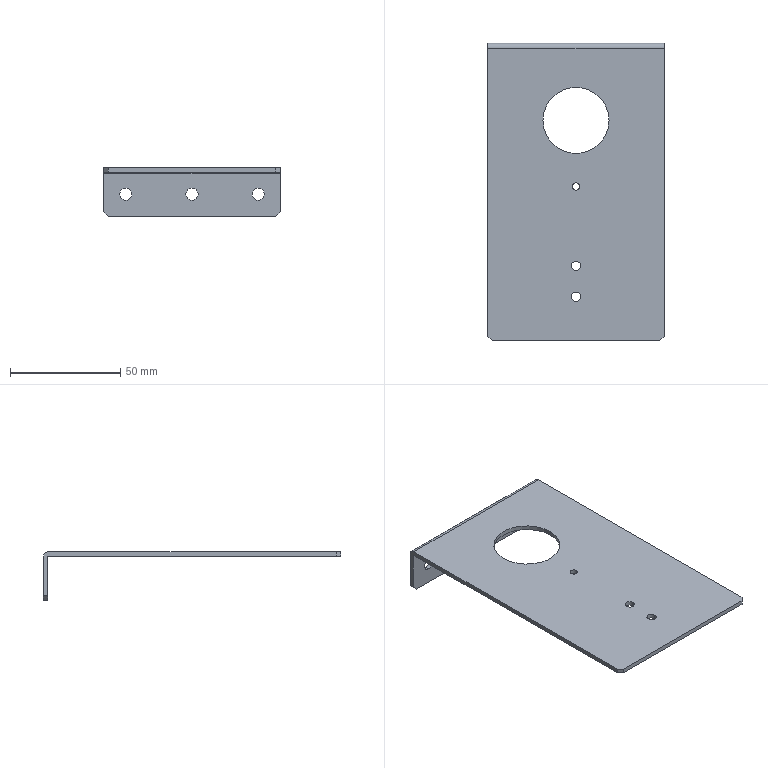Part | SolidWorks | features BaseBody 1 | 1 solid | 28 faces | box 80 x 135 x 22 mm | volume 23052 mm3 | cylinder 16 | plane 12 | commonest cylinder face diameters 5.5 x6 4.2 x4 3.3 x2 30 x2 1 x1 5 x1
STEP:
#1=CARTESIAN_POINT('',(37.9,34.,2.));
#2=VERTEX_POINT('',#1);
#3=CARTESIAN_POINT('',(42.1,34.,2.));
#4=VERTEX_POINT('',#3);
#5=CARTESIAN_POINT('',(40.,34.,2.));
#6=DIRECTION('',(0.,0.,1.));
#7=DIRECTION('',(-1.,0.,0.));
#8=AXIS2_PLACEMENT_3D('',#5,#6,#7);
#9=CIRCLE('',#8,2.1);
#10=EDGE_CURVE('',#2,#4,#9,.T.);
#11=ORIENTED_EDGE('',*,*,#10,.T.);
#12=CARTESIAN_POINT('',(42.1,34.,0.));
#13=VERTEX_POINT('',#12);
#14=CARTESIAN_POINT('',(42.1,34.,0.));
#15=DIRECTION('',(0.,0.,-1.));
#16=VECTOR('',#15,1000.);
#17=LINE('',#14,#16);
#18=EDGE_CURVE('',#4,#13,#17,.T.);
#19=ORIENTED_EDGE('',*,*,#18,.T.);
#20=CARTESIAN_POINT('',(37.9,34.,0.));
#21=VERTEX_POINT('',#20);
#22=CARTESIAN_POINT('',(40.,34.,0.));
#23=DIRECTION('',(0.,0.,1.));
#24=DIRECTION('',(-1.,0.,0.));
#25=AXIS2_PLACEMENT_3D('',#22,#23,#24);
#26=CIRCLE('',#25,2.1);
#27=EDGE_CURVE('',#21,#13,#26,.T.);
#28=ORIENTED_EDGE('',*,*,#27,.F.);
#29=CARTESIAN_POINT('',(37.9,34.,0.));
#30=DIRECTION('',(0.,0.,-1.));
#31=VECTOR('',#30,1000.);
#32=LINE('',#29,#31);
#33=EDGE_CURVE('',#2,#21,#32,.T.);
#34=ORIENTED_EDGE('',*,*,#33,.F.);
#35=EDGE_LOOP('',(#11,#19,#28,#34));
#36=FACE_OUTER_BOUND('',#35,.T.);
#37=CARTESIAN_POINT('',(40.,34.,0.));
#38=DIRECTION('',(0.,0.,-1.));
#39=DIRECTION('',(-1.,0.,0.));
#40=AXIS2_PLACEMENT_3D('',#37,#38,#39);
#41=CYLINDRICAL_SURFACE('',#40,2.1);
#42=ADVANCED_FACE('',(#36),#41,.F.);
#43=CARTESIAN_POINT('',(37.9,20.,2.));
#44=VERTEX_POINT('',#43);
#45=CARTESIAN_POINT('',(42.1,20.,2.));
#46=VERTEX_POINT('',#45);
#47=CARTESIAN_POINT('',(40.,20.,2.));
#48=DIRECTION('',(0.,0.,1.));
#49=DIRECTION('',(-1.,0.,0.));
#50=AXIS2_PLACEMENT_3D('',#47,#48,#49);
#51=CIRCLE('',#50,2.1);
#52=EDGE_CURVE('',#44,#46,#51,.T.);
#53=ORIENTED_EDGE('',*,*,#52,.T.);
#54=CARTESIAN_POINT('',(42.1,20.,0.));
#55=VERTEX_POINT('',#54);
#56=CARTESIAN_POINT('',(42.1,20.,0.));
#57=DIRECTION('',(0.,0.,-1.));
#58=VECTOR('',#57,1000.);
#59=LINE('',#56,#58);
#60=EDGE_CURVE('',#46,#55,#59,.T.);
#61=ORIENTED_EDGE('',*,*,#60,.T.);
#62=CARTESIAN_POINT('',(37.9,20.,0.));
#63=VERTEX_POINT('',#62);
#64=CARTESIAN_POINT('',(40.,20.,0.));
#65=DIRECTION('',(0.,0.,1.));
#66=DIRECTION('',(-1.,0.,0.));
#67=AXIS2_PLACEMENT_3D('',#64,#65,#66);
#68=CIRCLE('',#67,2.1);
#69=EDGE_CURVE('',#63,#55,#68,.T.);
#70=ORIENTED_EDGE('',*,*,#69,.F.);
#71=CARTESIAN_POINT('',(37.9,20.,0.));
#72=DIRECTION('',(0.,0.,-1.));
#73=VECTOR('',#72,1000.);
#74=LINE('',#71,#73);
#75=EDGE_CURVE('',#44,#63,#74,.T.);
#76=ORIENTED_EDGE('',*,*,#75,.F.);
#77=EDGE_LOOP('',(#53,#61,#70,#76));
#78=FACE_OUTER_BOUND('',#77,.T.);
#79=CARTESIAN_POINT('',(40.,20.,0.));
#80=DIRECTION('',(0.,0.,-1.));
#81=DIRECTION('',(-1.,0.,0.));
#82=AXIS2_PLACEMENT_3D('',#79,#80,#81);
#83=CYLINDRICAL_SURFACE('',#82,2.1);
#84=ADVANCED_FACE('',(#78),#83,.F.);
#85=CARTESIAN_POINT('',(25.,100.,2.));
#86=VERTEX_POINT('',#85);
#87=CARTESIAN_POINT('',(55.,100.,2.));
#88=VERTEX_POINT('',#87);
#89=CARTESIAN_POINT('',(40.,100.,2.));
#90=DIRECTION('',(0.,0.,1.));
#91=DIRECTION('',(-1.,0.,0.));
#92=AXIS2_PLACEMENT_3D('',#89,#90,#91);
#93=CIRCLE('',#92,15.);
#94=EDGE_CURVE('',#86,#88,#93,.T.);
#95=ORIENTED_EDGE('',*,*,#94,.T.);
#96=CARTESIAN_POINT('',(55.,100.,0.));
#97=VERTEX_POINT('',#96);
#98=CARTESIAN_POINT('',(55.,100.,10.));
#99=DIRECTION('',(0.,0.,-1.));
#100=VECTOR('',#99,1000.);
#101=LINE('',#98,#100);
#102=EDGE_CURVE('',#88,#97,#101,.T.);
#103=ORIENTED_EDGE('',*,*,#102,.T.);
#104=CARTESIAN_POINT('',(25.,100.,0.));
#105=VERTEX_POINT('',#104);
#106=CARTESIAN_POINT('',(40.,100.,0.));
#107=DIRECTION('',(0.,0.,1.));
#108=DIRECTION('',(-1.,0.,0.));
#109=AXIS2_PLACEMENT_3D('',#106,#107,#108);
#110=CIRCLE('',#109,15.);
#111=EDGE_CURVE('',#105,#97,#110,.T.);
#112=ORIENTED_EDGE('',*,*,#111,.F.);
#113=CARTESIAN_POINT('',(25.,100.,10.));
#114=DIRECTION('',(0.,0.,-1.));
#115=VECTOR('',#114,1000.);
#116=LINE('',#113,#115);
#117=EDGE_CURVE('',#86,#105,#116,.T.);
#118=ORIENTED_EDGE('',*,*,#117,.F.);
#119=EDGE_LOOP('',(#95,#103,#112,#118));
#120=FACE_OUTER_BOUND('',#119,.T.);
#121=CARTESIAN_POINT('',(40.,100.,10.));
#122=DIRECTION('',(0.,0.,-1.));
#123=DIRECTION('',(-1.,0.,0.));
#124=AXIS2_PLACEMENT_3D('',#121,#122,#123);
#125=CYLINDRICAL_SURFACE('',#124,15.);
#126=ADVANCED_FACE('',(#120),#125,.F.);
#127=CARTESIAN_POINT('',(38.35,70.,2.));
#128=VERTEX_POINT('',#127);
#129=CARTESIAN_POINT('',(41.65,70.,2.));
#130=VERTEX_POINT('',#129);
#131=CARTESIAN_POINT('',(40.,70.,2.));
#132=DIRECTION('',(0.,0.,1.));
#133=DIRECTION('',(-1.,0.,0.));
#134=AXIS2_PLACEMENT_3D('',#131,#132,#133);
#135=CIRCLE('',#134,1.65);
#136=EDGE_CURVE('',#128,#130,#135,.T.);
#137=ORIENTED_EDGE('',*,*,#136,.T.);
#138=CARTESIAN_POINT('',(41.65,70.,0.));
#139=VERTEX_POINT('',#138);
#140=CARTESIAN_POINT('',(41.65,70.,0.));
#141=DIRECTION('',(0.,0.,-1.));
#142=VECTOR('',#141,1000.);
#143=LINE('',#140,#142);
#144=EDGE_CURVE('',#130,#139,#143,.T.);
#145=ORIENTED_EDGE('',*,*,#144,.T.);
#146=CARTESIAN_POINT('',(38.35,70.,0.));
#147=VERTEX_POINT('',#146);
#148=CARTESIAN_POINT('',(40.,70.,0.));
#149=DIRECTION('',(0.,0.,1.));
#150=DIRECTION('',(-1.,0.,0.));
#151=AXIS2_PLACEMENT_3D('',#148,#149,#150);
#152=CIRCLE('',#151,1.65);
#153=EDGE_CURVE('',#147,#139,#152,.T.);
#154=ORIENTED_EDGE('',*,*,#153,.F.);
#155=CARTESIAN_POINT('',(38.35,70.,0.));
#156=DIRECTION('',(0.,0.,-1.));
#157=VECTOR('',#156,1000.);
#158=LINE('',#155,#157);
#159=EDGE_CURVE('',#128,#147,#158,.T.);
#160=ORIENTED_EDGE('',*,*,#159,.F.);
#161=EDGE_LOOP('',(#137,#145,#154,#160));
#162=FACE_OUTER_BOUND('',#161,.T.);
#163=CARTESIAN_POINT('',(40.,70.,0.));
#164=DIRECTION('',(0.,0.,-1.));
#165=DIRECTION('',(-1.,0.,0.));
#166=AXIS2_PLACEMENT_3D('',#163,#164,#165);
#167=CYLINDRICAL_SURFACE('',#166,1.65);
#168=ADVANCED_FACE('',(#162),#167,.F.);
#169=CARTESIAN_POINT('',(10.,135.,-12.75));
#170=VERTEX_POINT('',#169);
#171=CARTESIAN_POINT('',(10.,135.,-7.25));
#172=VERTEX_POINT('',#171);
#173=CARTESIAN_POINT('',(10.,135.,-10.));
#174=DIRECTION('',(0.,1.,0.));
#175=DIRECTION('',(0.,0.,-1.));
#176=AXIS2_PLACEMENT_3D('',#173,#174,#175);
#177=CIRCLE('',#176,2.75);
#178=EDGE_CURVE('',#170,#172,#177,.T.);
#179=ORIENTED_EDGE('',*,*,#178,.T.);
#180=CARTESIAN_POINT('',(10.,133.,-7.25));
#181=VERTEX_POINT('',#180);
#182=CARTESIAN_POINT('',(10.,133.,-7.25));
#183=DIRECTION('',(0.,-1.,0.));
#184=VECTOR('',#183,1000.);
#185=LINE('',#182,#184);
#186=EDGE_CURVE('',#172,#181,#185,.T.);
#187=ORIENTED_EDGE('',*,*,#186,.T.);
#188=CARTESIAN_POINT('',(10.,133.,-12.75));
#189=VERTEX_POINT('',#188);
#190=CARTESIAN_POINT('',(10.,133.,-10.));
#191=DIRECTION('',(0.,1.,0.));
#192=DIRECTION('',(0.,0.,-1.));
#193=AXIS2_PLACEMENT_3D('',#190,#191,#192);
#194=CIRCLE('',#193,2.75);
#195=EDGE_CURVE('',#189,#181,#194,.T.);
#196=ORIENTED_EDGE('',*,*,#195,.F.);
#197=CARTESIAN_POINT('',(10.,133.,-12.75));
#198=DIRECTION('',(0.,-1.,0.));
#199=VECTOR('',#198,1000.);
#200=LINE('',#197,#199);
#201=EDGE_CURVE('',#170,#189,#200,.T.);
#202=ORIENTED_EDGE('',*,*,#201,.F.);
#203=EDGE_LOOP('',(#179,#187,#196,#202));
#204=FACE_OUTER_BOUND('',#203,.T.);
#205=CARTESIAN_POINT('',(10.,133.,-10.));
#206=DIRECTION('',(0.,-1.,0.));
#207=DIRECTION('',(0.,0.,-1.));
#208=AXIS2_PLACEMENT_3D('',#205,#206,#207);
#209=CYLINDRICAL_SURFACE('',#208,2.75);
#210=ADVANCED_FACE('',(#204),#209,.F.);
#211=CARTESIAN_POINT('',(40.,135.,-12.75));
#212=VERTEX_POINT('',#211);
#213=CARTESIAN_POINT('',(40.,135.,-7.25));
#214=VERTEX_POINT('',#213);
#215=CARTESIAN_POINT('',(40.,135.,-10.));
#216=DIRECTION('',(0.,1.,0.));
#217=DIRECTION('',(0.,0.,-1.));
#218=AXIS2_PLACEMENT_3D('',#215,#216,#217);
#219=CIRCLE('',#218,2.75);
#220=EDGE_CURVE('',#212,#214,#219,.T.);
#221=ORIENTED_EDGE('',*,*,#220,.T.);
#222=CARTESIAN_POINT('',(40.,133.,-7.25));
#223=VERTEX_POINT('',#222);
#224=CARTESIAN_POINT('',(40.,133.,-7.25));
#225=DIRECTION('',(0.,-1.,0.));
#226=VECTOR('',#225,1000.);
#227=LINE('',#224,#226);
#228=EDGE_CURVE('',#214,#223,#227,.T.);
#229=ORIENTED_EDGE('',*,*,#228,.T.);
#230=CARTESIAN_POINT('',(40.,133.,-12.75));
#231=VERTEX_POINT('',#230);
#232=CARTESIAN_POINT('',(40.,133.,-10.));
#233=DIRECTION('',(0.,1.,0.));
#234=DIRECTION('',(0.,0.,-1.));
#235=AXIS2_PLACEMENT_3D('',#232,#233,#234);
#236=CIRCLE('',#235,2.75);
#237=EDGE_CURVE('',#231,#223,#236,.T.);
#238=ORIENTED_EDGE('',*,*,#237,.F.);
#239=CARTESIAN_POINT('',(40.,133.,-12.75));
#240=DIRECTION('',(0.,-1.,0.));
#241=VECTOR('',#240,1000.);
#242=LINE('',#239,#241);
#243=EDGE_CURVE('',#212,#231,#242,.T.);
#244=ORIENTED_EDGE('',*,*,#243,.F.);
#245=EDGE_LOOP('',(#221,#229,#238,#244));
#246=FACE_OUTER_BOUND('',#245,.T.);
#247=CARTESIAN_POINT('',(40.,133.,-10.));
#248=DIRECTION('',(0.,-1.,0.));
#249=DIRECTION('',(0.,0.,-1.));
#250=AXIS2_PLACEMENT_3D('',#247,#248,#249);
#251=CYLINDRICAL_SURFACE('',#250,2.75);
#252=ADVANCED_FACE('',(#246),#251,.F.);
#253=CARTESIAN_POINT('',(70.,135.,-12.75));
#254=VERTEX_POINT('',#253);
#255=CARTESIAN_POINT('',(70.,135.,-7.25));
#256=VERTEX_POINT('',#255);
#257=CARTESIAN_POINT('',(70.,135.,-10.));
#258=DIRECTION('',(0.,1.,0.));
#259=DIRECTION('',(0.,0.,-1.));
#260=AXIS2_PLACEMENT_3D('',#257,#258,#259);
#261=CIRCLE('',#260,2.75);
#262=EDGE_CURVE('',#254,#256,#261,.T.);
#263=ORIENTED_EDGE('',*,*,#262,.T.);
#264=CARTESIAN_POINT('',(70.,133.,-7.25));
#265=VERTEX_POINT('',#264);
#266=CARTESIAN_POINT('',(70.,133.,-7.25));
#267=DIRECTION('',(0.,-1.,0.));
#268=VECTOR('',#267,1000.);
#269=LINE('',#266,#268);
#270=EDGE_CURVE('',#256,#265,#269,.T.);
#271=ORIENTED_EDGE('',*,*,#270,.T.);
#272=CARTESIAN_POINT('',(70.,133.,-12.75));
#273=VERTEX_POINT('',#272);
#274=CARTESIAN_POINT('',(70.,133.,-10.));
#275=DIRECTION('',(0.,1.,0.));
#276=DIRECTION('',(0.,0.,-1.));
#277=AXIS2_PLACEMENT_3D('',#274,#275,#276);
#278=CIRCLE('',#277,2.75);
#279=EDGE_CURVE('',#273,#265,#278,.T.);
#280=ORIENTED_EDGE('',*,*,#279,.F.);
#281=CARTESIAN_POINT('',(70.,133.,-12.75));
#282=DIRECTION('',(0.,-1.,0.));
#283=VECTOR('',#282,1000.);
#284=LINE('',#281,#283);
#285=EDGE_CURVE('',#254,#273,#284,.T.);
#286=ORIENTED_EDGE('',*,*,#285,.F.);
#287=EDGE_LOOP('',(#263,#271,#280,#286));
#288=FACE_OUTER_BOUND('',#287,.T.);
#289=CARTESIAN_POINT('',(70.,133.,-10.));
#290=DIRECTION('',(0.,-1.,0.));
#291=DIRECTION('',(0.,0.,-1.));
#292=AXIS2_PLACEMENT_3D('',#289,#290,#291);
#293=CYLINDRICAL_SURFACE('',#292,2.75);
#294=ADVANCED_FACE('',(#288),#293,.F.);
#295=CARTESIAN_POINT('',(2.,0.,2.));
#296=VERTEX_POINT('',#295);
#297=CARTESIAN_POINT('',(0.,2.,2.));
#298=VERTEX_POINT('',#297);
#299=CARTESIAN_POINT('',(2.,0.,2.));
#300=DIRECTION('',(-0.7071,0.7071,0.));
#301=VECTOR('',#300,1000.);
#302=LINE('',#299,#301);
#303=EDGE_CURVE('',#296,#298,#302,.T.);
#304=ORIENTED_EDGE('',*,*,#303,.F.);
#305=CARTESIAN_POINT('',(78.,0.,2.));
#306=VERTEX_POINT('',#305);
#307=CARTESIAN_POINT('',(0.,0.,2.));
#308=DIRECTION('',(-1.,0.,0.));
#309=VECTOR('',#308,1000.);
#310=LINE('',#307,#309);
#311=EDGE_CURVE('',#306,#296,#310,.T.);
#312=ORIENTED_EDGE('',*,*,#311,.F.);
#313=CARTESIAN_POINT('',(80.,2.,2.));
#314=VERTEX_POINT('',#313);
#315=CARTESIAN_POINT('',(80.,2.,2.));
#316=DIRECTION('',(-0.7071,-0.7071,0.));
#317=VECTOR('',#316,1000.);
#318=LINE('',#315,#317);
#319=EDGE_CURVE('',#314,#306,#318,.T.);
#320=ORIENTED_EDGE('',*,*,#319,.F.);
#321=CARTESIAN_POINT('',(80.,132.5,2.));
#322=VERTEX_POINT('',#321);
#323=CARTESIAN_POINT('',(80.,135.,2.));
#324=DIRECTION('',(0.,-1.,0.));
#325=VECTOR('',#324,1000.);
#326=LINE('',#323,#325);
#327=EDGE_CURVE('',#322,#314,#326,.T.);
#328=ORIENTED_EDGE('',*,*,#327,.F.);
#329=CARTESIAN_POINT('',(0.,132.5,2.));
#330=VERTEX_POINT('',#329);
#331=CARTESIAN_POINT('',(0.,132.5,2.));
#332=DIRECTION('',(1.,0.,0.));
#333=VECTOR('',#332,1000.);
#334=LINE('',#331,#333);
#335=EDGE_CURVE('',#330,#322,#334,.T.);
#336=ORIENTED_EDGE('',*,*,#335,.F.);
#337=CARTESIAN_POINT('',(0.,135.,2.));
#338=DIRECTION('',(0.,1.,0.));
#339=VECTOR('',#338,1000.);
#340=LINE('',#337,#339);
#341=EDGE_CURVE('',#298,#330,#340,.T.);
#342=ORIENTED_EDGE('',*,*,#341,.F.);
#343=EDGE_LOOP('',(#304,#312,#320,#328,#336,#342));
#344=FACE_OUTER_BOUND('',#343,.T.);
#345=ORIENTED_EDGE('',*,*,#10,.F.);
#346=CARTESIAN_POINT('',(40.,34.,2.));
#347=DIRECTION('',(0.,0.,1.));
#348=DIRECTION('',(-1.,0.,0.));
#349=AXIS2_PLACEMENT_3D('',#346,#347,#348);
#350=CIRCLE('',#349,2.1);
#351=EDGE_CURVE('',#4,#2,#350,.T.);
#352=ORIENTED_EDGE('',*,*,#351,.F.);
#353=EDGE_LOOP('',(#345,#352));
#354=FACE_BOUND('',#353,.T.);
#355=ORIENTED_EDGE('',*,*,#52,.F.);
#356=CARTESIAN_POINT('',(40.,20.,2.));
#357=DIRECTION('',(0.,0.,1.));
#358=DIRECTION('',(-1.,0.,0.));
#359=AXIS2_PLACEMENT_3D('',#356,#357,#358);
#360=CIRCLE('',#359,2.1);
#361=EDGE_CURVE('',#46,#44,#360,.T.);
#362=ORIENTED_EDGE('',*,*,#361,.F.);
#363=EDGE_LOOP('',(#355,#362));
#364=FACE_BOUND('',#363,.T.);
#365=ORIENTED_EDGE('',*,*,#94,.F.);
#366=CARTESIAN_POINT('',(40.,100.,2.));
#367=DIRECTION('',(0.,0.,1.));
#368=DIRECTION('',(-1.,0.,0.));
#369=AXIS2_PLACEMENT_3D('',#366,#367,#368);
#370=CIRCLE('',#369,15.);
#371=EDGE_CURVE('',#88,#86,#370,.T.);
#372=ORIENTED_EDGE('',*,*,#371,.F.);
#373=EDGE_LOOP('',(#365,#372));
#374=FACE_BOUND('',#373,.T.);
#375=ORIENTED_EDGE('',*,*,#136,.F.);
#376=CARTESIAN_POINT('',(40.,70.,2.));
#377=DIRECTION('',(0.,0.,1.));
#378=DIRECTION('',(-1.,0.,0.));
#379=AXIS2_PLACEMENT_3D('',#376,#377,#378);
#380=CIRCLE('',#379,1.65);
#381=EDGE_CURVE('',#130,#128,#380,.T.);
#382=ORIENTED_EDGE('',*,*,#381,.F.);
#383=EDGE_LOOP('',(#375,#382));
#384=FACE_BOUND('',#383,.T.);
#385=CARTESIAN_POINT('',(0.,135.,2.));
#386=DIRECTION('',(0.,0.,-1.));
#387=DIRECTION('',(-1.,0.,0.));
#388=AXIS2_PLACEMENT_3D('',#385,#386,#387);
#389=PLANE('',#388);
#390=ADVANCED_FACE('',(#344,#354,#364,#374,#384),#389,.F.);
#391=ORIENTED_EDGE('',*,*,#341,.T.);
#392=CARTESIAN_POINT('',(0.,135.,-0.5));
#393=VERTEX_POINT('',#392);
#394=CARTESIAN_POINT('',(0.,132.5,-0.5));
#395=DIRECTION('',(1.,0.,0.));
#396=DIRECTION('',(0.,0.,-1.));
#397=AXIS2_PLACEMENT_3D('',#394,#395,#396);
#398=CIRCLE('',#397,2.5);
#399=EDGE_CURVE('',#393,#330,#398,.T.);
#400=ORIENTED_EDGE('',*,*,#399,.F.);
#401=CARTESIAN_POINT('',(0.,135.,-18.));
#402=VERTEX_POINT('',#401);
#403=CARTESIAN_POINT('',(0.,135.,0.));
#404=DIRECTION('',(0.,0.,-1.));
#405=VECTOR('',#404,1000.);
#406=LINE('',#403,#405);
#407=EDGE_CURVE('',#393,#402,#406,.T.);
#408=ORIENTED_EDGE('',*,*,#407,.T.);
#409=CARTESIAN_POINT('',(0.,133.,-18.));
#410=VERTEX_POINT('',#409);
#411=CARTESIAN_POINT('',(0.,135.,-18.));
#412=DIRECTION('',(0.,1.,0.));
#413=VECTOR('',#412,1000.);
#414=LINE('',#411,#413);
#415=EDGE_CURVE('',#410,#402,#414,.T.);
#416=ORIENTED_EDGE('',*,*,#415,.F.);
#417=CARTESIAN_POINT('',(0.,133.,-0.5));
#418=VERTEX_POINT('',#417);
#419=CARTESIAN_POINT('',(0.,133.,0.));
#420=DIRECTION('',(0.,0.,-1.));
#421=VECTOR('',#420,1000.);
#422=LINE('',#419,#421);
#423=EDGE_CURVE('',#418,#410,#422,.T.);
#424=ORIENTED_EDGE('',*,*,#423,.F.);
#425=CARTESIAN_POINT('',(0.,132.5,0.));
#426=VERTEX_POINT('',#425);
#427=CARTESIAN_POINT('',(0.,132.5,-0.5));
#428=DIRECTION('',(1.,0.,0.));
#429=DIRECTION('',(0.,0.,-1.));
#430=AXIS2_PLACEMENT_3D('',#427,#428,#429);
#431=CIRCLE('',#430,0.5);
#432=EDGE_CURVE('',#418,#426,#431,.T.);
#433=ORIENTED_EDGE('',*,*,#432,.T.);
#434=CARTESIAN_POINT('',(0.,2.,0.));
#435=VERTEX_POINT('',#434);
#436=CARTESIAN_POINT('',(0.,135.,0.));
#437=DIRECTION('',(0.,-1.,0.));
#438=VECTOR('',#437,1000.);
#439=LINE('',#436,#438);
#440=EDGE_CURVE('',#426,#435,#439,.T.);
#441=ORIENTED_EDGE('',*,*,#440,.T.);
#442=CARTESIAN_POINT('',(0.,2.,2.));
#443=DIRECTION('',(0.,0.,1.));
#444=VECTOR('',#443,1000.);
#445=LINE('',#442,#444);
#446=EDGE_CURVE('',#435,#298,#445,.T.);
#447=ORIENTED_EDGE('',*,*,#446,.T.);
#448=EDGE_LOOP('',(#391,#400,#408,#416,#424,#433,#441,#447));
#449=FACE_OUTER_BOUND('',#448,.T.);
#450=CARTESIAN_POINT('',(0.,135.,2.));
#451=DIRECTION('',(-1.,0.,0.));
#452=DIRECTION('',(0.,0.,1.));
#453=AXIS2_PLACEMENT_3D('',#450,#451,#452);
#454=PLANE('',#453);
#455=ADVANCED_FACE('',(#449),#454,.T.);
#456=ORIENTED_EDGE('',*,*,#446,.F.);
#457=CARTESIAN_POINT('',(2.,0.,0.));
#458=VERTEX_POINT('',#457);
#459=CARTESIAN_POINT('',(2.,0.,0.));
#460=DIRECTION('',(-0.7071,0.7071,0.));
#461=VECTOR('',#460,1000.);
#462=LINE('',#459,#461);
#463=EDGE_CURVE('',#458,#435,#462,.T.);
#464=ORIENTED_EDGE('',*,*,#463,.F.);
#465=CARTESIAN_POINT('',(2.,0.,0.));
#466=DIRECTION('',(0.,0.,-1.));
#467=VECTOR('',#466,1000.);
#468=LINE('',#465,#467);
#469=EDGE_CURVE('',#296,#458,#468,.T.);
#470=ORIENTED_EDGE('',*,*,#469,.F.);
#471=ORIENTED_EDGE('',*,*,#303,.T.);
#472=EDGE_LOOP('',(#456,#464,#470,#471));
#473=FACE_OUTER_BOUND('',#472,.T.);
#474=CARTESIAN_POINT('',(2.,0.,0.));
#475=DIRECTION('',(0.7071,0.7071,0.));
#476=DIRECTION('',(-0.7071,0.7071,0.));
#477=AXIS2_PLACEMENT_3D('',#474,#475,#476);
#478=PLANE('',#477);
#479=ADVANCED_FACE('',(#473),#478,.F.);
#480=CARTESIAN_POINT('',(78.,0.,0.));
#481=VERTEX_POINT('',#480);
#482=CARTESIAN_POINT('',(0.,0.,0.));
#483=DIRECTION('',(1.,0.,0.));
#484=VECTOR('',#483,1000.);
#485=LINE('',#482,#484);
#486=EDGE_CURVE('',#458,#481,#485,.T.);
#487=ORIENTED_EDGE('',*,*,#486,.T.);
#488=CARTESIAN_POINT('',(78.,0.,0.));
#489=DIRECTION('',(0.,0.,1.));
#490=VECTOR('',#489,1000.);
#491=LINE('',#488,#490);
#492=EDGE_CURVE('',#481,#306,#491,.T.);
#493=ORIENTED_EDGE('',*,*,#492,.T.);
#494=ORIENTED_EDGE('',*,*,#311,.T.);
#495=ORIENTED_EDGE('',*,*,#469,.T.);
#496=EDGE_LOOP('',(#487,#493,#494,#495));
#497=FACE_OUTER_BOUND('',#496,.T.);
#498=CARTESIAN_POINT('',(0.,0.,0.));
#499=DIRECTION('',(0.,-1.,0.));
#500=DIRECTION('',(0.,0.,-1.));
#501=AXIS2_PLACEMENT_3D('',#498,#499,#500);
#502=PLANE('',#501);
#503=ADVANCED_FACE('',(#497),#502,.T.);
#504=CARTESIAN_POINT('',(80.,2.,0.));
#505=VERTEX_POINT('',#504);
#506=CARTESIAN_POINT('',(80.,2.,0.));
#507=DIRECTION('',(0.,0.,-1.));
#508=VECTOR('',#507,1000.);
#509=LINE('',#506,#508);
#510=EDGE_CURVE('',#314,#505,#509,.T.);
#511=ORIENTED_EDGE('',*,*,#510,.F.);
#512=ORIENTED_EDGE('',*,*,#319,.T.);
#513=ORIENTED_EDGE('',*,*,#492,.F.);
#514=CARTESIAN_POINT('',(78.,0.,0.));
#515=DIRECTION('',(-0.7071,-0.7071,0.));
#516=VECTOR('',#515,1000.);
#517=LINE('',#514,#516);
#518=EDGE_CURVE('',#505,#481,#517,.T.);
#519=ORIENTED_EDGE('',*,*,#518,.F.);
#520=EDGE_LOOP('',(#511,#512,#513,#519));
#521=FACE_OUTER_BOUND('',#520,.T.);
#522=CARTESIAN_POINT('',(78.,0.,0.));
#523=DIRECTION('',(-0.7071,0.7071,0.));
#524=DIRECTION('',(-0.7071,-0.7071,0.));
#525=AXIS2_PLACEMENT_3D('',#522,#523,#524);
#526=PLANE('',#525);
#527=ADVANCED_FACE('',(#521),#526,.F.);
#528=CARTESIAN_POINT('',(80.,132.5,0.));
#529=VERTEX_POINT('',#528);
#530=CARTESIAN_POINT('',(80.,135.,0.));
#531=DIRECTION('',(0.,1.,0.));
#532=VECTOR('',#531,1000.);
#533=LINE('',#530,#532);
#534=EDGE_CURVE('',#505,#529,#533,.T.);
#535=ORIENTED_EDGE('',*,*,#534,.T.);
#536=CARTESIAN_POINT('',(80.,133.,-0.5));
#537=VERTEX_POINT('',#536);
#538=CARTESIAN_POINT('',(80.,132.5,-0.5));
#539=DIRECTION('',(1.,0.,0.));
#540=DIRECTION('',(0.,0.,-1.));
#541=AXIS2_PLACEMENT_3D('',#538,#539,#540);
#542=CIRCLE('',#541,0.5);
#543=EDGE_CURVE('',#537,#529,#542,.T.);
#544=ORIENTED_EDGE('',*,*,#543,.F.);
#545=CARTESIAN_POINT('',(80.,133.,-18.));
#546=VERTEX_POINT('',#545);
#547=CARTESIAN_POINT('',(80.,133.,-20.));
#548=DIRECTION('',(0.,0.,1.));
#549=VECTOR('',#548,1000.);
#550=LINE('',#547,#549);
#551=EDGE_CURVE('',#546,#537,#550,.T.);
#552=ORIENTED_EDGE('',*,*,#551,.F.);
#553=CARTESIAN_POINT('',(80.,135.,-18.));
#554=VERTEX_POINT('',#553);
#555=CARTESIAN_POINT('',(80.,135.,-18.));
#556=DIRECTION('',(0.,-1.,0.));
#557=VECTOR('',#556,1000.);
#558=LINE('',#555,#557);
#559=EDGE_CURVE('',#554,#546,#558,.T.);
#560=ORIENTED_EDGE('',*,*,#559,.F.);
#561=CARTESIAN_POINT('',(80.,135.,-0.5));
#562=VERTEX_POINT('',#561);
#563=CARTESIAN_POINT('',(80.,135.,0.));
#564=DIRECTION('',(0.,0.,1.));
#565=VECTOR('',#564,1000.);
#566=LINE('',#563,#565);
#567=EDGE_CURVE('',#554,#562,#566,.T.);
#568=ORIENTED_EDGE('',*,*,#567,.T.);
#569=CARTESIAN_POINT('',(80.,132.5,-0.5));
#570=DIRECTION('',(-1.,0.,0.));
#571=DIRECTION('',(0.,0.,-1.));
#572=AXIS2_PLACEMENT_3D('',#569,#570,#571);
#573=CIRCLE('',#572,2.5);
#574=EDGE_CURVE('',#322,#562,#573,.T.);
#575=ORIENTED_EDGE('',*,*,#574,.F.);
#576=ORIENTED_EDGE('',*,*,#327,.T.);
#577=ORIENTED_EDGE('',*,*,#510,.T.);
#578=EDGE_LOOP('',(#535,#544,#552,#560,#568,#575,#576,#577));
#579=FACE_OUTER_BOUND('',#578,.T.);
#580=CARTESIAN_POINT('',(80.,135.,0.));
#581=DIRECTION('',(1.,0.,0.));
#582=DIRECTION('',(0.,0.,-1.));
#583=AXIS2_PLACEMENT_3D('',#580,#581,#582);
#584=PLANE('',#583);
#585=ADVANCED_FACE('',(#579),#584,.T.);
#586=CARTESIAN_POINT('',(80.,135.,-0.5));
#587=DIRECTION('',(-1.,0.,0.));
#588=VECTOR('',#587,1000.);
#589=LINE('',#586,#588);
#590=EDGE_CURVE('',#562,#393,#589,.T.);
#591=ORIENTED_EDGE('',*,*,#590,.T.);
#592=ORIENTED_EDGE('',*,*,#399,.T.);
#593=ORIENTED_EDGE('',*,*,#335,.T.);
#594=ORIENTED_EDGE('',*,*,#574,.T.);
#595=EDGE_LOOP('',(#591,#592,#593,#594));
#596=FACE_OUTER_BOUND('',#595,.T.);
#597=CARTESIAN_POINT('',(80.,132.5,-0.5));
#598=DIRECTION('',(1.,0.,0.));
#599=DIRECTION('',(0.,0.,-1.));
#600=AXIS2_PLACEMENT_3D('',#597,#598,#599);
#601=CYLINDRICAL_SURFACE('',#600,2.5);
#602=ADVANCED_FACE('',(#596),#601,.T.);
#603=ORIENTED_EDGE('',*,*,#18,.F.);
#604=ORIENTED_EDGE('',*,*,#351,.T.);
#605=ORIENTED_EDGE('',*,*,#33,.T.);
#606=CARTESIAN_POINT('',(40.,34.,0.));
#607=DIRECTION('',(0.,0.,1.));
#608=DIRECTION('',(-1.,0.,0.));
#609=AXIS2_PLACEMENT_3D('',#606,#607,#608);
#610=CIRCLE('',#609,2.1);
#611=EDGE_CURVE('',#13,#21,#610,.T.);
#612=ORIENTED_EDGE('',*,*,#611,.F.);
#613=EDGE_LOOP('',(#603,#604,#605,#612));
#614=FACE_OUTER_BOUND('',#613,.T.);
#615=CARTESIAN_POINT('',(40.,34.,0.));
#616=DIRECTION('',(0.,0.,-1.));
#617=DIRECTION('',(-1.,0.,0.));
#618=AXIS2_PLACEMENT_3D('',#615,#616,#617);
#619=CYLINDRICAL_SURFACE('',#618,2.1);
#620=ADVANCED_FACE('',(#614),#619,.F.);
#621=ORIENTED_EDGE('',*,*,#60,.F.);
#622=ORIENTED_EDGE('',*,*,#361,.T.);
#623=ORIENTED_EDGE('',*,*,#75,.T.);
#624=CARTESIAN_POINT('',(40.,20.,0.));
#625=DIRECTION('',(0.,0.,1.));
#626=DIRECTION('',(-1.,0.,0.));
#627=AXIS2_PLACEMENT_3D('',#624,#625,#626);
#628=CIRCLE('',#627,2.1);
#629=EDGE_CURVE('',#55,#63,#628,.T.);
#630=ORIENTED_EDGE('',*,*,#629,.F.);
#631=EDGE_LOOP('',(#621,#622,#623,#630));
#632=FACE_OUTER_BOUND('',#631,.T.);
#633=CARTESIAN_POINT('',(40.,20.,0.));
#634=DIRECTION('',(0.,0.,-1.));
#635=DIRECTION('',(-1.,0.,0.));
#636=AXIS2_PLACEMENT_3D('',#633,#634,#635);
#637=CYLINDRICAL_SURFACE('',#636,2.1);
#638=ADVANCED_FACE('',(#632),#637,.F.);
#639=ORIENTED_EDGE('',*,*,#102,.F.);
#640=ORIENTED_EDGE('',*,*,#371,.T.);
#641=ORIENTED_EDGE('',*,*,#117,.T.);
#642=CARTESIAN_POINT('',(40.,100.,0.));
#643=DIRECTION('',(0.,0.,1.));
#644=DIRECTION('',(-1.,0.,0.));
#645=AXIS2_PLACEMENT_3D('',#642,#643,#644);
#646=CIRCLE('',#645,15.);
#647=EDGE_CURVE('',#97,#105,#646,.T.);
#648=ORIENTED_EDGE('',*,*,#647,.F.);
#649=EDGE_LOOP('',(#639,#640,#641,#648));
#650=FACE_OUTER_BOUND('',#649,.T.);
#651=CARTESIAN_POINT('',(40.,100.,10.));
#652=DIRECTION('',(0.,0.,-1.));
#653=DIRECTION('',(-1.,0.,0.));
#654=AXIS2_PLACEMENT_3D('',#651,#652,#653);
#655=CYLINDRICAL_SURFACE('',#654,15.);
#656=ADVANCED_FACE('',(#650),#655,.F.);
#657=ORIENTED_EDGE('',*,*,#144,.F.);
#658=ORIENTED_EDGE('',*,*,#381,.T.);
#659=ORIENTED_EDGE('',*,*,#159,.T.);
#660=CARTESIAN_POINT('',(40.,70.,0.));
#661=DIRECTION('',(0.,0.,1.));
#662=DIRECTION('',(-1.,0.,0.));
#663=AXIS2_PLACEMENT_3D('',#660,#661,#662);
#664=CIRCLE('',#663,1.65);
#665=EDGE_CURVE('',#139,#147,#664,.T.);
#666=ORIENTED_EDGE('',*,*,#665,.F.);
#667=EDGE_LOOP('',(#657,#658,#659,#666));
#668=FACE_OUTER_BOUND('',#667,.T.);
#669=CARTESIAN_POINT('',(40.,70.,0.));
#670=DIRECTION('',(0.,0.,-1.));
#671=DIRECTION('',(-1.,0.,0.));
#672=AXIS2_PLACEMENT_3D('',#669,#670,#671);
#673=CYLINDRICAL_SURFACE('',#672,1.65);
#674=ADVANCED_FACE('',(#668),#673,.F.);
#675=ORIENTED_EDGE('',*,*,#534,.F.);
#676=ORIENTED_EDGE('',*,*,#518,.T.);
#677=ORIENTED_EDGE('',*,*,#486,.F.);
#678=ORIENTED_EDGE('',*,*,#463,.T.);
#679=ORIENTED_EDGE('',*,*,#440,.F.);
#680=CARTESIAN_POINT('',(0.,132.5,0.));
#681=DIRECTION('',(1.,0.,0.));
#682=VECTOR('',#681,1000.);
#683=LINE('',#680,#682);
#684=EDGE_CURVE('',#426,#529,#683,.T.);
#685=ORIENTED_EDGE('',*,*,#684,.T.);
#686=EDGE_LOOP('',(#675,#676,#677,#678,#679,#685));
#687=FACE_OUTER_BOUND('',#686,.T.);
#688=ORIENTED_EDGE('',*,*,#69,.T.);
#689=ORIENTED_EDGE('',*,*,#629,.T.);
#690=EDGE_LOOP('',(#688,#689));
#691=FACE_BOUND('',#690,.T.);
#692=ORIENTED_EDGE('',*,*,#27,.T.);
#693=ORIENTED_EDGE('',*,*,#611,.T.);
#694=EDGE_LOOP('',(#692,#693));
#695=FACE_BOUND('',#694,.T.);
#696=ORIENTED_EDGE('',*,*,#111,.T.);
#697=ORIENTED_EDGE('',*,*,#647,.T.);
#698=EDGE_LOOP('',(#696,#697));
#699=FACE_BOUND('',#698,.T.);
#700=ORIENTED_EDGE('',*,*,#153,.T.);
#701=ORIENTED_EDGE('',*,*,#665,.T.);
#702=EDGE_LOOP('',(#700,#701));
#703=FACE_BOUND('',#702,.T.);
#704=CARTESIAN_POINT('',(0.,135.,0.));
#705=DIRECTION('',(0.,0.,-1.));
#706=DIRECTION('',(-1.,0.,0.));
#707=AXIS2_PLACEMENT_3D('',#704,#705,#706);
#708=PLANE('',#707);
#709=ADVANCED_FACE('',(#687,#691,#695,#699,#703),#708,.T.);
#710=CARTESIAN_POINT('',(78.,135.,-20.));
#711=VERTEX_POINT('',#710);
#712=CARTESIAN_POINT('',(78.,135.,-20.));
#713=DIRECTION('',(0.7071,0.,0.7071));
#714=VECTOR('',#713,1000.);
#715=LINE('',#712,#714);
#716=EDGE_CURVE('',#711,#554,#715,.T.);
#717=ORIENTED_EDGE('',*,*,#716,.F.);
#718=CARTESIAN_POINT('',(2.,135.,-20.));
#719=VERTEX_POINT('',#718);
#720=CARTESIAN_POINT('',(0.,135.,-20.));
#721=DIRECTION('',(1.,0.,0.));
#722=VECTOR('',#721,1000.);
#723=LINE('',#720,#722);
#724=EDGE_CURVE('',#719,#711,#723,.T.);
#725=ORIENTED_EDGE('',*,*,#724,.F.);
#726=CARTESIAN_POINT('',(0.,135.,-18.));
#727=DIRECTION('',(0.7071,0.,-0.7071));
#728=VECTOR('',#727,1000.);
#729=LINE('',#726,#728);
#730=EDGE_CURVE('',#402,#719,#729,.T.);
#731=ORIENTED_EDGE('',*,*,#730,.F.);
#732=ORIENTED_EDGE('',*,*,#407,.F.);
#733=ORIENTED_EDGE('',*,*,#590,.F.);
#734=ORIENTED_EDGE('',*,*,#567,.F.);
#735=EDGE_LOOP('',(#717,#725,#731,#732,#733,#734));
#736=FACE_OUTER_BOUND('',#735,.T.);
#737=ORIENTED_EDGE('',*,*,#178,.F.);
#738=CARTESIAN_POINT('',(10.,135.,-10.));
#739=DIRECTION('',(0.,1.,0.));
#740=DIRECTION('',(0.,0.,-1.));
#741=AXIS2_PLACEMENT_3D('',#738,#739,#740);
#742=CIRCLE('',#741,2.75);
#743=EDGE_CURVE('',#172,#170,#742,.T.);
#744=ORIENTED_EDGE('',*,*,#743,.F.);
#745=EDGE_LOOP('',(#737,#744));
#746=FACE_BOUND('',#745,.T.);
#747=ORIENTED_EDGE('',*,*,#220,.F.);
#748=CARTESIAN_POINT('',(40.,135.,-10.));
#749=DIRECTION('',(0.,1.,0.));
#750=DIRECTION('',(0.,0.,-1.));
#751=AXIS2_PLACEMENT_3D('',#748,#749,#750);
#752=CIRCLE('',#751,2.75);
#753=EDGE_CURVE('',#214,#212,#752,.T.);
#754=ORIENTED_EDGE('',*,*,#753,.F.);
#755=EDGE_LOOP('',(#747,#754));
#756=FACE_BOUND('',#755,.T.);
#757=ORIENTED_EDGE('',*,*,#262,.F.);
#758=CARTESIAN_POINT('',(70.,135.,-10.));
#759=DIRECTION('',(0.,1.,0.));
#760=DIRECTION('',(0.,0.,-1.));
#761=AXIS2_PLACEMENT_3D('',#758,#759,#760);
#762=CIRCLE('',#761,2.75);
#763=EDGE_CURVE('',#256,#254,#762,.T.);
#764=ORIENTED_EDGE('',*,*,#763,.F.);
#765=EDGE_LOOP('',(#757,#764));
#766=FACE_BOUND('',#765,.T.);
#767=CARTESIAN_POINT('',(0.,135.,0.));
#768=DIRECTION('',(0.,-1.,0.));
#769=DIRECTION('',(0.,0.,-1.));
#770=AXIS2_PLACEMENT_3D('',#767,#768,#769);
#771=PLANE('',#770);
#772=ADVANCED_FACE('',(#736,#746,#756,#766),#771,.F.);
#773=ORIENTED_EDGE('',*,*,#432,.F.);
#774=CARTESIAN_POINT('',(80.,133.,-0.5));
#775=DIRECTION('',(-1.,0.,0.));
#776=VECTOR('',#775,1000.);
#777=LINE('',#774,#776);
#778=EDGE_CURVE('',#537,#418,#777,.T.);
#779=ORIENTED_EDGE('',*,*,#778,.F.);
#780=ORIENTED_EDGE('',*,*,#543,.T.);
#781=ORIENTED_EDGE('',*,*,#684,.F.);
#782=EDGE_LOOP('',(#773,#779,#780,#781));
#783=FACE_OUTER_BOUND('',#782,.T.);
#784=CARTESIAN_POINT('',(80.,132.5,-0.5));
#785=DIRECTION('',(1.,0.,0.));
#786=DIRECTION('',(0.,0.,-1.));
#787=AXIS2_PLACEMENT_3D('',#784,#785,#786);
#788=CYLINDRICAL_SURFACE('',#787,0.5);
#789=ADVANCED_FACE('',(#783),#788,.F.);
#790=ORIENTED_EDGE('',*,*,#559,.T.);
#791=CARTESIAN_POINT('',(78.,133.,-20.));
#792=VERTEX_POINT('',#791);
#793=CARTESIAN_POINT('',(78.,133.,-20.));
#794=DIRECTION('',(0.7071,0.,0.7071));
#795=VECTOR('',#794,1000.);
#796=LINE('',#793,#795);
#797=EDGE_CURVE('',#792,#546,#796,.T.);
#798=ORIENTED_EDGE('',*,*,#797,.F.);
#799=CARTESIAN_POINT('',(78.,135.,-20.));
#800=DIRECTION('',(0.,-1.,0.));
#801=VECTOR('',#800,1000.);
#802=LINE('',#799,#801);
#803=EDGE_CURVE('',#711,#792,#802,.T.);
#804=ORIENTED_EDGE('',*,*,#803,.F.);
#805=ORIENTED_EDGE('',*,*,#716,.T.);
#806=EDGE_LOOP('',(#790,#798,#804,#805));
#807=FACE_OUTER_BOUND('',#806,.T.);
#808=CARTESIAN_POINT('',(78.,135.,-20.));
#809=DIRECTION('',(-0.7071,0.,0.7071));
#810=DIRECTION('',(0.7071,0.,0.7071));
#811=AXIS2_PLACEMENT_3D('',#808,#809,#810);
#812=PLANE('',#811);
#813=ADVANCED_FACE('',(#807),#812,.F.);
#814=ORIENTED_EDGE('',*,*,#803,.T.);
#815=CARTESIAN_POINT('',(2.,133.,-20.));
#816=VERTEX_POINT('',#815);
#817=CARTESIAN_POINT('',(0.,133.,-20.));
#818=DIRECTION('',(1.,0.,0.));
#819=VECTOR('',#818,1000.);
#820=LINE('',#817,#819);
#821=EDGE_CURVE('',#816,#792,#820,.T.);
#822=ORIENTED_EDGE('',*,*,#821,.F.);
#823=CARTESIAN_POINT('',(2.,135.,-20.));
#824=DIRECTION('',(0.,-1.,0.));
#825=VECTOR('',#824,1000.);
#826=LINE('',#823,#825);
#827=EDGE_CURVE('',#719,#816,#826,.T.);
#828=ORIENTED_EDGE('',*,*,#827,.F.);
#829=ORIENTED_EDGE('',*,*,#724,.T.);
#830=EDGE_LOOP('',(#814,#822,#828,#829));
#831=FACE_OUTER_BOUND('',#830,.T.);
#832=CARTESIAN_POINT('',(0.,135.,-20.));
#833=DIRECTION('',(0.,0.,1.));
#834=DIRECTION('',(0.,-1.,0.));
#835=AXIS2_PLACEMENT_3D('',#832,#833,#834);
#836=PLANE('',#835);
#837=ADVANCED_FACE('',(#831),#836,.F.);
#838=ORIENTED_EDGE('',*,*,#827,.T.);
#839=CARTESIAN_POINT('',(0.,133.,-18.));
#840=DIRECTION('',(0.7071,0.,-0.7071));
#841=VECTOR('',#840,1000.);
#842=LINE('',#839,#841);
#843=EDGE_CURVE('',#410,#816,#842,.T.);
#844=ORIENTED_EDGE('',*,*,#843,.F.);
#845=ORIENTED_EDGE('',*,*,#415,.T.);
#846=ORIENTED_EDGE('',*,*,#730,.T.);
#847=EDGE_LOOP('',(#838,#844,#845,#846));
#848=FACE_OUTER_BOUND('',#847,.T.);
#849=CARTESIAN_POINT('',(0.,135.,-18.));
#850=DIRECTION('',(0.7071,0.,0.7071));
#851=DIRECTION('',(0.7071,0.,-0.7071));
#852=AXIS2_PLACEMENT_3D('',#849,#850,#851);
#853=PLANE('',#852);
#854=ADVANCED_FACE('',(#848),#853,.F.);
#855=ORIENTED_EDGE('',*,*,#186,.F.);
#856=ORIENTED_EDGE('',*,*,#743,.T.);
#857=ORIENTED_EDGE('',*,*,#201,.T.);
#858=CARTESIAN_POINT('',(10.,133.,-10.));
#859=DIRECTION('',(0.,1.,0.));
#860=DIRECTION('',(0.,0.,-1.));
#861=AXIS2_PLACEMENT_3D('',#858,#859,#860);
#862=CIRCLE('',#861,2.75);
#863=EDGE_CURVE('',#181,#189,#862,.T.);
#864=ORIENTED_EDGE('',*,*,#863,.F.);
#865=EDGE_LOOP('',(#855,#856,#857,#864));
#866=FACE_OUTER_BOUND('',#865,.T.);
#867=CARTESIAN_POINT('',(10.,133.,-10.));
#868=DIRECTION('',(0.,-1.,0.));
#869=DIRECTION('',(0.,0.,-1.));
#870=AXIS2_PLACEMENT_3D('',#867,#868,#869);
#871=CYLINDRICAL_SURFACE('',#870,2.75);
#872=ADVANCED_FACE('',(#866),#871,.F.);
#873=ORIENTED_EDGE('',*,*,#228,.F.);
#874=ORIENTED_EDGE('',*,*,#753,.T.);
#875=ORIENTED_EDGE('',*,*,#243,.T.);
#876=CARTESIAN_POINT('',(40.,133.,-10.));
#877=DIRECTION('',(0.,1.,0.));
#878=DIRECTION('',(0.,0.,-1.));
#879=AXIS2_PLACEMENT_3D('',#876,#877,#878);
#880=CIRCLE('',#879,2.75);
#881=EDGE_CURVE('',#223,#231,#880,.T.);
#882=ORIENTED_EDGE('',*,*,#881,.F.);
#883=EDGE_LOOP('',(#873,#874,#875,#882));
#884=FACE_OUTER_BOUND('',#883,.T.);
#885=CARTESIAN_POINT('',(40.,133.,-10.));
#886=DIRECTION('',(0.,-1.,0.));
#887=DIRECTION('',(0.,0.,-1.));
#888=AXIS2_PLACEMENT_3D('',#885,#886,#887);
#889=CYLINDRICAL_SURFACE('',#888,2.75);
#890=ADVANCED_FACE('',(#884),#889,.F.);
#891=ORIENTED_EDGE('',*,*,#270,.F.);
#892=ORIENTED_EDGE('',*,*,#763,.T.);
#893=ORIENTED_EDGE('',*,*,#285,.T.);
#894=CARTESIAN_POINT('',(70.,133.,-10.));
#895=DIRECTION('',(0.,1.,0.));
#896=DIRECTION('',(0.,0.,-1.));
#897=AXIS2_PLACEMENT_3D('',#894,#895,#896);
#898=CIRCLE('',#897,2.75);
#899=EDGE_CURVE('',#265,#273,#898,.T.);
#900=ORIENTED_EDGE('',*,*,#899,.F.);
#901=EDGE_LOOP('',(#891,#892,#893,#900));
#902=FACE_OUTER_BOUND('',#901,.T.);
#903=CARTESIAN_POINT('',(70.,133.,-10.));
#904=DIRECTION('',(0.,-1.,0.));
#905=DIRECTION('',(0.,0.,-1.));
#906=AXIS2_PLACEMENT_3D('',#903,#904,#905);
#907=CYLINDRICAL_SURFACE('',#906,2.75);
#908=ADVANCED_FACE('',(#902),#907,.F.);
#909=ORIENTED_EDGE('',*,*,#423,.T.);
#910=ORIENTED_EDGE('',*,*,#843,.T.);
#911=ORIENTED_EDGE('',*,*,#821,.T.);
#912=ORIENTED_EDGE('',*,*,#797,.T.);
#913=ORIENTED_EDGE('',*,*,#551,.T.);
#914=ORIENTED_EDGE('',*,*,#778,.T.);
#915=EDGE_LOOP('',(#909,#910,#911,#912,#913,#914));
#916=FACE_OUTER_BOUND('',#915,.T.);
#917=ORIENTED_EDGE('',*,*,#195,.T.);
#918=ORIENTED_EDGE('',*,*,#863,.T.);
#919=EDGE_LOOP('',(#917,#918));
#920=FACE_BOUND('',#919,.T.);
#921=ORIENTED_EDGE('',*,*,#237,.T.);
#922=ORIENTED_EDGE('',*,*,#881,.T.);
#923=EDGE_LOOP('',(#921,#922));
#924=FACE_BOUND('',#923,.T.);
#925=ORIENTED_EDGE('',*,*,#279,.T.);
#926=ORIENTED_EDGE('',*,*,#899,.T.);
#927=EDGE_LOOP('',(#925,#926));
#928=FACE_BOUND('',#927,.T.);
#929=CARTESIAN_POINT('',(0.,133.,0.));
#930=DIRECTION('',(0.,-1.,0.));
#931=DIRECTION('',(0.,0.,-1.));
#932=AXIS2_PLACEMENT_3D('',#929,#930,#931);
#933=PLANE('',#932);
#934=ADVANCED_FACE('',(#916,#920,#924,#928),#933,.T.);
#935=CLOSED_SHELL('',(#42,#84,#126,#168,#210,#252,#294,#390,#455,#479,#503,#527,#585,#602,#620,#638,#656,#674,#709,#772,#789,#813,#837,#854,#872,#890,#908,#934));
#936=MANIFOLD_SOLID_BREP('',#935);
#937=CARTESIAN_POINT('',(0.,0.,0.));
#938=DIRECTION('',(0.,0.,1.));
#939=DIRECTION('',(1.,0.,0.));
#940=AXIS2_PLACEMENT_3D('',#937,#938,#939);
#941=(LENGTH_UNIT()NAMED_UNIT(*)SI_UNIT(.MILLI.,.METRE.));
#942=UNCERTAINTY_MEASURE_WITH_UNIT(LENGTH_MEASURE(0.00001),#941,'','');
#943=(NAMED_UNIT(*)PLANE_ANGLE_UNIT()SI_UNIT($,.RADIAN.));
#944=(NAMED_UNIT(*)SI_UNIT($,.STERADIAN.)SOLID_ANGLE_UNIT());
#945=(GEOMETRIC_REPRESENTATION_CONTEXT(3)GLOBAL_UNCERTAINTY_ASSIGNED_CONTEXT((#942))GLOBAL_UNIT_ASSIGNED_CONTEXT((#941,#943,#944))REPRESENTATION_CONTEXT('',''));
#946=ADVANCED_BREP_SHAPE_REPRESENTATION('',(#936,#940),#945);